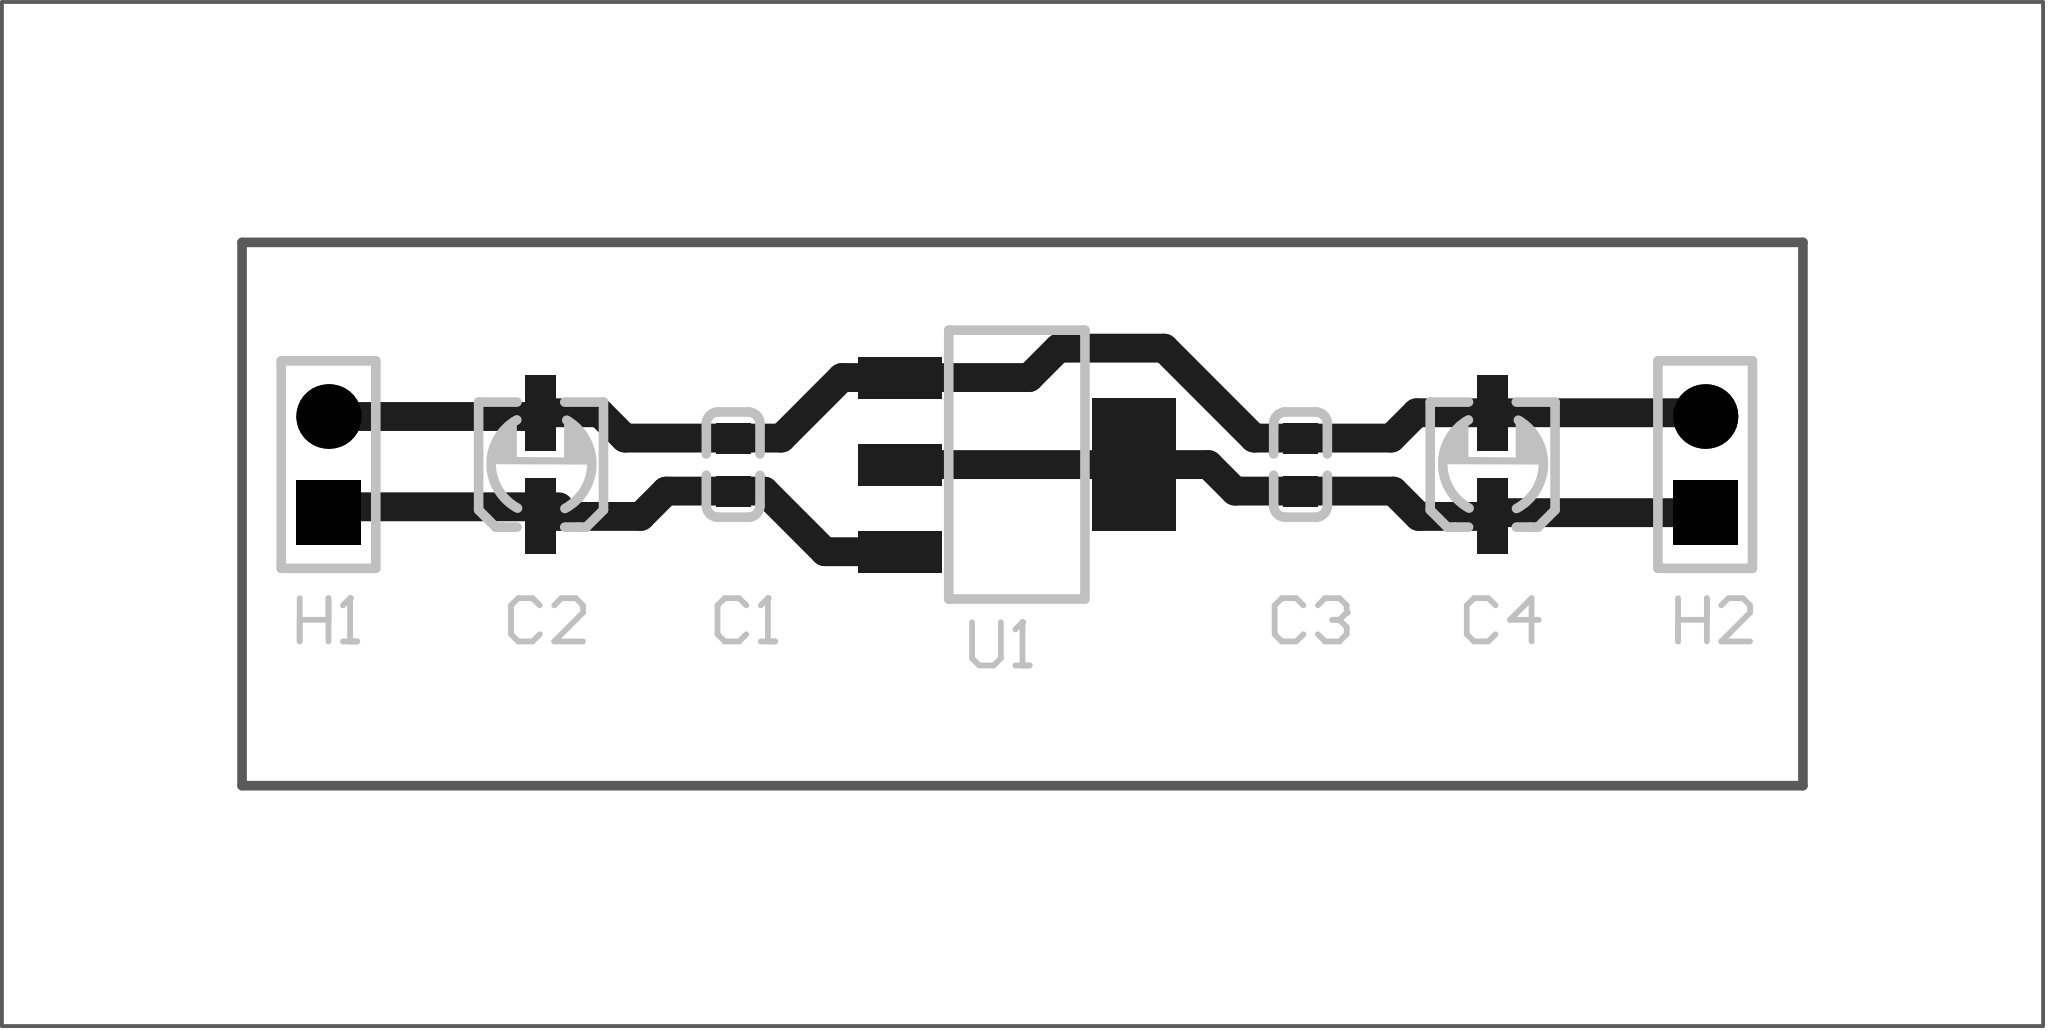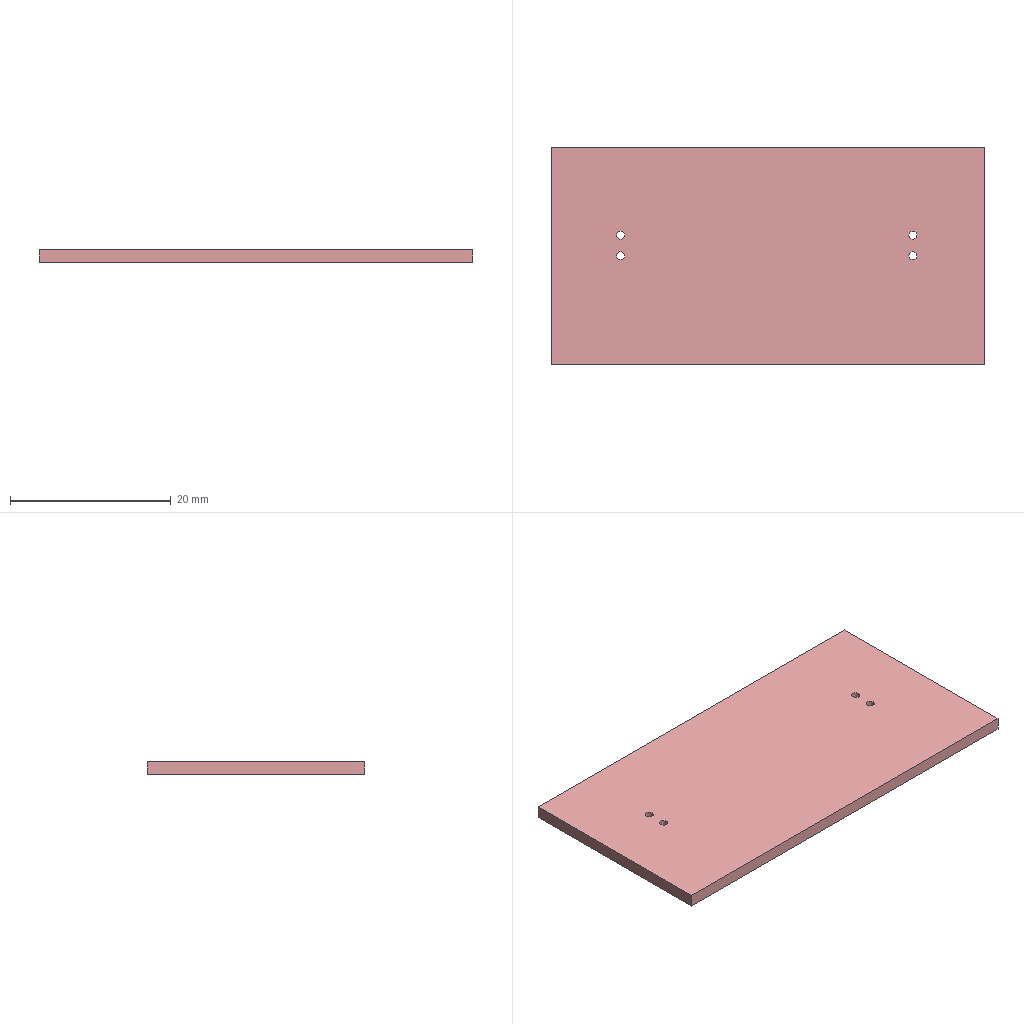Circuit board layout | Altium Designer | box 54 x 27.1 x 1.6 mm
Layer stack:
# Altium Designer layer stack of  (unit mm; dielectric type: 0 none, 1 core, 2 prepreg, 3 surface material)
index,name,kind,layer,copper_thickness_mm,dielectric_type,dielectric_thickness_mm,dielectric_material,dielectric_constant
0,Top Paste Mask Layer,other,,,,,,
1,Top Silkscreen Layer,other,,,,,,
2,Top Solder Mask Layer,dielectric,,,3,0.01,,3.3
3,Top Layer,copper,Top Layer,0.035,,,,
4,Dielectric1,dielectric,,,3,1.51,FR4,4.5
5,Bottom Layer,copper,Bottom Layer,0.035,,,,
6,Bottom Solder Mask Layer,dielectric,,,3,0.01,,3.3
7,Bottom Silkscreen Layer,other,,,,,,
8,Bottom Paste Mask Layer,other,,,,,,
# drill layer pairs: low layer,high layer
drill_pair,Top Layer,Bottom Layer
Part placement:
Designator,Comment,Layer,Footprint,Center-X(mm),Center-Y(mm),Rotation
C1,100nF,TopLayer,C0603,89.187,84.681,270
C2,10uF,TopLayer,C_Ele_SMD_3x5.4mm,84.101,84.681,270
C3,100nF,TopLayer,C0603,104.189,84.681,270
C4,10uF,TopLayer,C_Ele_SMD_3x5.4mm,109.264,84.681,270
H1,,TopLayer,HDR-TH_2P-P2.54-V-F,78.486,84.681,90
H2,,TopLayer,HDR-TH_2P-P2.54-V-F,114.89,84.681,90
U1,,TopLayer,SOT_223,96.688,84.68,270
Pad and via stacks:
# Altium Designer via and pad stacks of  (unit mm). Each distinct definition once, with the count of objects using it.
# via: kind,start_layer,end_layer,hole_mm,diameter_mm,mode(0 simple;1 top-mid-bottom;2 full stack),diameter_per_layer,count,example_net
# pad: kind,layer,hole_mm,hole_type(0 round;1 square;2 slot),plating,top_size,top_shape(1 round;2 rect;3 octagon;9 rounded rect),mid_size,bottom_size,mode,footprint,size_per_layer,count,example
pad,Top Layer,0,0,plated,0.8x0.9,2,0.8x0.9,0.8x0.9,0,C0603,,4,C1.2
pad,Top Layer,0,0,plated,1.999x0.8001,2,1.999x0.8001,1.999x0.8001,0,C_Ele_SMD_3x5.4mm,,4,C2.1
pad,Top Layer,0,0,plated,2.2x3.5,2,2.2x3.5,2.2x3.5,0,SOT_223,,1,U1.4
pad,Top Layer,0,0,plated,1.1x2.2,2,1.1x2.2,1.1x2.2,0,SOT_223,,3,U1.3
pad,Multi-Layer,1,0,plated,1.7x1.7,2,1.7x1.7,1.7x1.7,0,HDR-TH_2P-P2.54-V-F,,2,H1.1
pad,Multi-Layer,1,0,plated,1.7x1.7,1,1.7x1.7,1.7x1.7,0,HDR-TH_2P-P2.54-V-F,,2,H1.2